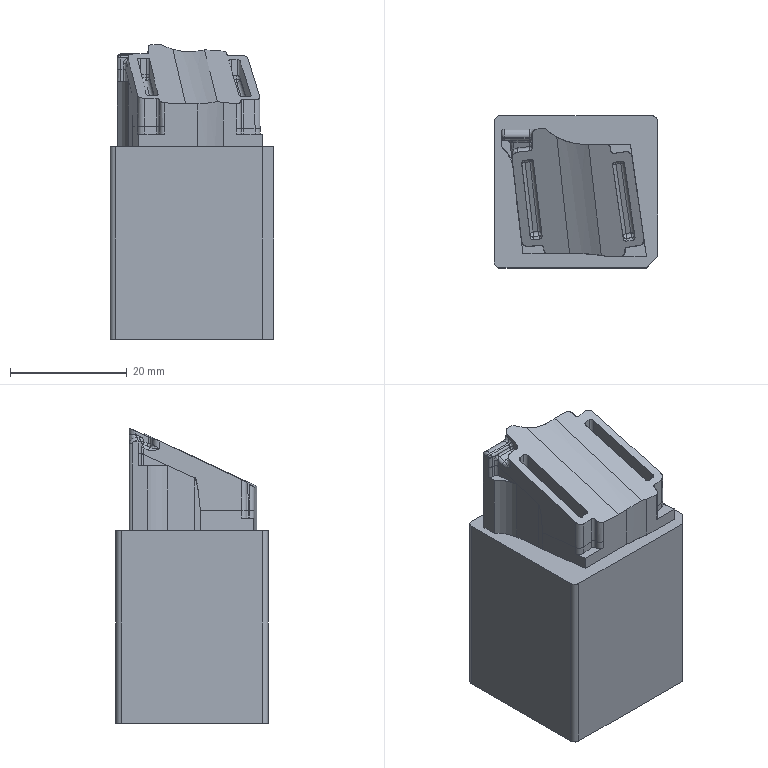NC program | NX | posted with a generic post | part box 28 x 26 x 50.455 mm
Lines 1 to 1159 of 12518:
N10 G17 G21 G94 G90
(ZLEVEL_PROFILE_COPY , TOOL : D0.5)
N12 T00 M6
N14 G54
N16 G17 G0 G90 X-7.188 Y11.048 S0 M3
N18 G43 Z10. H0
N20 Z0.198
N22 G94 G1 Z-0.102 F250.
N24 G3 X-6.499 Y10.968 R3.
N26 G1 X-5.218
N28 X-5.116 Y10.979
N30 X-5.049 Y10.902
N32 X-4.947 Y10.81
N34 G3 X-4.652 Y10.578 R3.
N36 G1 Z0.198
N38 G0 Z0.997
N40 X-4.451 Y10.419
N42 Z0.098
N44 G1 Z-0.202
N46 G2 X-4.773 Y10.658 R3.
N48 X-5.049 Y10.902 R9.75
N50 G1 X-5.116 Y10.979
N52 X-5.218 Y10.968
N54 X-6.5
N56 G2 X-7.189 Y11.048 R3.
N58 G1 Z0.098
N60 G0 Z0.898
N62 X-7.19
N64 Z-0.001
N66 G1 Z-0.301
N68 G3 X-6.5 Y10.968 R3.
N70 G1 X-5.218
N72 X-5.116 Y10.979
N74 X-5.049 Y10.902
N76 G3 X-4.553 Y10.476 R9.75
N78 X-4.22 Y10.244 R3.
N80 G1 Z-0.001
N82 G0 Z0.798
N84 X-3.978 Y10.072
N86 Z-0.1
N88 G1 Z-0.4
N90 G2 X-4.319 Y10.294 R3.
N92 X-5.049 Y10.902 R9.75
N94 G1 X-5.116 Y10.979
N96 X-5.218 Y10.968
N98 X-6.501
N100 G2 X-7.192 Y11.048 R3.
N102 G1 Z-0.1
N104 G0 Z0.699
N106 X-7.193
N108 Z-0.2
N110 G1 Z-0.5
N112 G3 X-6.501 Y10.968 R3.
N114 G1 X-5.218
N116 X-5.116 Y10.979
N118 X-5.049 Y10.902
N120 G3 X-4.07 Y10.112 R9.75
N122 X-3.726 Y9.903 R3.
N124 G1 Z-0.2
N126 G0 Z0.6
N128 X-3.456 Y9.735
N130 Z-0.299
N132 G1 Z-0.599
N134 G2 X-3.81 Y9.935 R3.
N136 X-4.07 Y10.112 R9.75
N138 X-5.049 Y10.902 R9.75
N140 G1 X-5.116 Y10.979
N142 X-5.218 Y10.968
N144 X-6.501
N146 G2 X-7.194 Y11.048 R3.
N148 G1 Z-0.299
N150 G0 Z0.5
N152 Z-0.398
N154 G1 Z-0.698
N156 G3 X-6.502 Y10.968 R3.
N158 G1 X-5.218
N160 X-5.116 Y10.979
N162 X-5.049 Y10.902
N164 G3 X-4.07 Y10.112 R9.75
N166 X-3.531 Y9.759 R9.75
N168 X-3.171 Y9.571 R3.
N170 G1 Z-0.398
N172 G0 Z0.401
N174 X-2.857 Y9.405
N176 Z-0.498
N178 G1 Z-0.798
N180 G2 X-3.233 Y9.584 R3.
N182 X-3.531 Y9.759 R9.75
N184 X-4.07 Y10.112 R9.75
N186 X-5.049 Y10.902 R9.75
N188 G1 X-5.116 Y10.979
N190 X-5.218 Y10.968
N192 X-6.501
N194 G2 X-7.195 Y11.048 R3.
N196 G1 Z-0.498
N198 G0 Z0.302
N200 Z-0.597
N202 G1 Z-0.897
N204 G3 X-6.504 Y10.968 R3.
N206 G1 X-5.218
N208 X-5.116 Y10.979
N210 X-5.049 Y10.902
N212 G3 X-4.07 Y10.112 R9.75
N214 X-3.531 Y9.759 R9.75
N216 X-3.233 Y9.584 R9.75
N218 G1 X-3.232 Y9.583
N220 G3 X-2.901 Y9.405 R9.75
N222 X-2.521 Y9.243 R3.
N224 G1 Z-0.597
N226 G0 Z0.202
N228 X-2.115 Y9.069
N230 Z-0.696
N232 G1 Z-0.996
N234 G2 X-2.52 Y9.22 R3.
N236 X-3.232 Y9.583 R9.75
N238 G1 X-3.233 Y9.584
N240 G2 X-3.531 Y9.759 R9.75
N242 X-4.07 Y10.112 R9.75
N244 X-5.049 Y10.902 R9.75
N246 G1 X-5.116 Y10.979
N248 X-5.218 Y10.968
N250 X-6.501
N252 X-6.506
N254 G2 X-7.198 Y11.048 R3.
N256 G1 Z-0.696
N258 G0 Z0.103
N260 X-7.214 Y11.051
N262 Z-0.796
N264 G1 Z-1.096
N266 G3 X-6.513 Y10.968 R3.
N268 G1 X-6.504
N270 X-5.218
N272 X-5.116 Y10.979
N274 X-5.049 Y10.902
N276 G3 X-4.07 Y10.112 R9.75
N278 X-3.233 Y9.584 R9.75
N280 G1 X-3.232 Y9.583
N282 G3 X-2.52 Y9.22 R9.75
N284 G1 X-2.478 Y9.201
N286 G3 X-2.054 Y9.021 R9.75
N288 X-1.664 Y8.896 R3.
N290 G1 Z-0.796
N292 G0 Z0.004
N294 X-1.126 Y8.713
N296 Z-0.895
N298 G1 Z-1.195
N300 G2 X-1.372 Y8.779 R3.
N302 X-2.054 Y9.021 R9.75
N304 X-2.478 Y9.201 R9.75
N306 G1 X-2.52 Y9.22
N308 G2 X-3.232 Y9.583 R9.75
N310 G1 X-3.233 Y9.584
N312 G2 X-4.07 Y10.112 R9.75
N314 X-5.049 Y10.902 R9.75
N316 G1 X-5.116 Y10.979
N318 X-5.218 Y10.968
N320 X-6.501
N322 X-6.513
N324 X-6.521
N326 G2 X-7.217 Y11.054 R3.
N328 G1 Z-0.895
N330 G0 Z10.
N332 X1.377 Y8.359
N334 Z-0.696
N336 G1 Z-0.996
N338 G3 X1.781 Y8.331 R3.
N340 G1 X3.342
N342 G3 X3.757 Y8.36 R3.
N344 G1 Z-0.696
N346 G0 Z0.103
N348 X5.252
N350 Z-0.796
N352 G1 Z-1.096
N354 G2 X4.837 Y8.331 R3.
N356 G1 X1.548
N358 G2 X1.309 Y8.334 R9.75
N360 X0.889 Y8.374 R3.
N362 G1 Z-0.796
N364 G0 Z0.004
N366 X0.234 Y8.439
N368 Z-0.895
N370 G1 Z-1.195
N372 G3 X0.635 Y8.374 R3.
N374 X1.294 Y8.334 R9.75
N376 G1 X1.309
N378 G3 X1.548 Y8.331 R9.75
N380 G1 X5.128
N382 G2 X5.669 Y8.174 R1.142
N384 G3 X6.037 Y7.99 R3.
N386 G1 Z-0.895
N388 G0 Z-0.096
N390 X6.22 Y7.666
N392 Z-0.994
N394 G1 Z-1.294
N396 G2 X5.901 Y7.985 R3.
N398 G3 X5.129 Y8.331 R0.992
N400 G1 X1.548
N402 G2 X1.309 Y8.334 R9.75
N404 G1 X1.294
N406 G2 X-2.054 Y9.021 R9.75
N408 X-2.478 Y9.201 R9.75
N410 G1 X-2.52 Y9.22
N412 G2 X-3.232 Y9.583 R9.75
N414 G1 X-3.233 Y9.584
N416 G2 X-4.07 Y10.112 R9.75
N418 X-5.049 Y10.902 R9.75
N420 G1 X-5.116 Y10.979
N422 X-5.218 Y10.968
N424 X-6.501
N426 X-6.513
N428 X-6.536
N430 X-6.538
N432 G2 X-7.255 Y11.052 R3.
N434 G1 Z-0.994
N436 G0 Z-0.195
N438 X-7.261 Y11.057
N440 Z-1.094
N442 G1 Z-1.394
N444 G3 X-6.559 Y10.968 R3.
N446 G1 X-6.541
N448 X-6.536
N450 X-6.513
N452 X-6.504
N454 X-5.218
N456 X-5.116 Y10.979
N458 X-5.049 Y10.902
N460 G3 X-4.07 Y10.112 R9.75
N462 X-3.233 Y9.584 R9.75
N464 G1 X-3.232 Y9.583
N466 G3 X-2.52 Y9.22 R9.75
N468 G1 X-2.478 Y9.201
N470 G3 X-2.054 Y9.021 R9.75
N472 X1.294 Y8.334 R9.75
N474 G1 X1.309
N476 G3 X1.548 Y8.331 R9.75
N478 G1 X5.129
N480 G2 X5.438 Y8.288 R0.992
N482 X6.002 Y7.856 R1.008
N484 G3 X6.346 Y7.563 R3.
N486 G1 Z-1.094
N488 G0 Z-0.294
N490 X6.24 Y6.997
N492 Z-1.193
N494 G1 Z-1.493
N496 G2 X6.166 Y7.405 R3.
N498 G3 X6.096 Y7.681 R1.042
N500 G1 X6.091 Y7.786
N502 X6.008 Y7.851
N504 X5.947 Y7.936
N506 G3 X5.438 Y8.288 R1.008
N508 X5.129 Y8.331 R0.992
N510 G1 X1.548
N512 G2 X1.309 Y8.334 R9.75
N514 G1 X1.294
N516 G2 X-2.054 Y9.021 R9.75
N518 X-2.478 Y9.201 R9.75
N520 G1 X-2.52 Y9.22
N522 G2 X-3.232 Y9.583 R9.75
N524 G1 X-3.233 Y9.584
N526 G2 X-4.07 Y10.112 R9.75
N528 X-5.049 Y10.902 R9.75
N530 G1 X-5.116 Y10.979
N532 X-5.218 Y10.968
N534 X-6.501
N536 X-6.513
N538 X-6.536
N540 X-6.541
N542 X-6.587
N544 G2 X-7.338 Y11.052 R3.
N546 G1 Z-1.193
N548 G0 Z-0.394
N550 X-7.351 Y11.065
N552 Z-1.292
N554 G1 Z-1.592
N556 G3 X-6.621 Y10.968 R3.
N558 G1 X-6.591
N560 X-6.541
N562 X-6.536
N564 X-6.513
N566 X-6.504
N568 X-5.218
N570 X-5.116 Y10.979
N572 X-5.049 Y10.902
N574 G3 X-4.07 Y10.112 R9.75
N576 X-3.233 Y9.584 R9.75
N578 G1 X-3.232 Y9.583
N580 G3 X-2.52 Y9.22 R9.75
N582 G1 X-2.478 Y9.201
N584 G3 X-2.054 Y9.021 R9.75
N586 X1.294 Y8.334 R9.75
N588 G1 X1.309
N590 G3 X1.548 Y8.331 R9.75
N592 G1 X5.129
N594 G2 X5.438 Y8.288 R0.992
N596 X5.834 Y8.061 R1.008
N598 X6.022 Y7.835 R1.05
N600 G1 X6.09 Y7.789
N602 Y7.707
N604 G2 X6.18 Y7.279 R1.05
N606 G1 Y7.118
N608 G3 X6.204 Y6.733 R3.
N610 G1 Z-1.292
N612 G0 Z-0.493
N614 X6.218 Y6.555
N616 Z-1.391
N618 G1 Z-1.691
N620 G2 X6.18 Y7.04 R3.
N622 G1 X6.181 Y7.279
N624 G3 X6.089 Y7.71 R1.05
N626 G1 X6.09 Y7.789
N628 X6.024 Y7.833
N630 G3 X5.817 Y8.076 R1.05
N632 X5.438 Y8.288 R1.008
N634 X5.129 Y8.331 R0.992
N636 G1 X1.548
N638 G2 X1.309 Y8.334 R9.75
N640 G1 X1.294
N642 G2 X-2.054 Y9.021 R9.75
N644 X-2.478 Y9.201 R9.75
N646 G1 X-2.52 Y9.22
N648 G2 X-3.232 Y9.583 R9.75
N650 G1 X-3.233 Y9.584
N652 G2 X-4.07 Y10.112 R9.75
N654 X-5.049 Y10.902 R9.75
N656 G1 X-5.116 Y10.979
N658 X-5.218 Y10.968
N660 X-6.501
N662 X-6.513
N664 X-6.536
N666 X-6.541
N668 X-6.591
N670 X-6.66
N672 G2 X-7.421 Y11.049 R3.
N674 G1 Z-1.391
N676 G0 Z-0.592
N678 X-7.471 Y11.066
N680 Z-1.491
N682 G1 Z-1.791
N684 G3 X-6.71 Y10.968 R3.
N686 G1 X-6.676
N688 X-6.591
N690 X-6.541
N692 X-6.536
N694 X-6.513
N696 X-6.504
N698 X-5.218
N700 X-5.116 Y10.979
N702 X-5.049 Y10.902
N704 G3 X-4.07 Y10.112 R9.75
N706 X-3.233 Y9.584 R9.75
N708 G1 X-3.232 Y9.583
N710 G3 X-2.52 Y9.22 R9.75
N712 G1 X-2.478 Y9.201
N714 G3 X-2.054 Y9.021 R9.75
N716 X1.294 Y8.334 R9.75
N718 G1 X1.309
N720 G3 X1.548 Y8.331 R9.75
N722 G1 X5.129
N724 G2 X5.438 Y8.288 R0.992
N726 X5.801 Y8.09 R1.008
N728 X6.026 Y7.831 R1.05
N730 G1 X6.09 Y7.789
N732 X6.088 Y7.713
N734 G2 X6.181 Y7.279 R1.05
N736 G1 Y7.083
N738 G3 X6.247 Y6.885 R0.526
N740 X6.482 Y6.537 R3.
N742 G1 Z-1.491
N744 G0 Z-0.691
N746 X6.785 Y6.691
N748 Z-1.59
N750 G1 Z-1.89
N752 G2 X6.37 Y6.811 R3.
N754 G1 X6.267 Y6.836
N756 X6.223 Y6.932
N758 X6.181 Y7.079
N760 Y7.083
N762 X6.182 Y7.279
N764 G3 X6.087 Y7.716 R1.05
N766 G1 X6.028 Y7.829
N768 G3 X5.784 Y8.104 R1.05
N770 X5.438 Y8.288 R1.008
N772 X5.129 Y8.331 R0.992
N774 G1 X1.548
N776 G2 X1.309 Y8.334 R9.75
N778 G1 X1.294
N780 G2 X-2.054 Y9.021 R9.75
N782 X-2.478 Y9.201 R9.75
N784 G1 X-2.52 Y9.22
N786 G2 X-3.232 Y9.583 R9.75
N788 G1 X-3.233 Y9.584
N790 G2 X-4.07 Y10.112 R9.75
N792 X-5.049 Y10.902 R9.75
N794 G1 X-5.116 Y10.979
N796 X-5.218 Y10.968
N798 X-6.501
N800 X-6.513
N802 X-6.536
N804 X-6.541
N806 X-6.591
N808 X-6.676
N810 X-6.764
N812 G2 X-7.545 Y11.071 R3.
N814 G1 Z-1.59
N816 G0 Z-0.791
N818 X-7.645 Y11.08
N820 Z-1.689
N822 G1 Z-1.989
N824 G3 X-6.832 Y10.968 R3.
N826 G1 X-6.764
N828 X-6.676
N830 X-6.591
N832 X-6.541
N834 X-6.536
N836 X-6.513
N838 X-6.504
N840 X-5.218
N842 X-5.116 Y10.979
N844 X-5.049 Y10.902
N846 G3 X-4.07 Y10.112 R9.75
N848 X-3.233 Y9.584 R9.75
N850 G1 X-3.232 Y9.583
N852 G3 X-2.52 Y9.22 R9.75
N854 G1 X-2.478 Y9.201
N856 G3 X-2.054 Y9.021 R9.75
N858 X1.294 Y8.334 R9.75
N860 G1 X1.309
N862 G3 X1.548 Y8.331 R9.75
N864 G1 X5.129
N866 G2 X5.438 Y8.288 R0.992
N868 X5.766 Y8.118 R1.008
N870 X6.03 Y7.826 R1.05
N872 G1 X6.086 Y7.72
N874 G2 X6.182 Y7.279 R1.05
N876 G1 Y7.083
N878 X6.181 Y7.078
N880 X6.223 Y6.932
N882 X6.267 Y6.836
N884 X6.37 Y6.811
N886 X6.389 Y6.804
N888 X6.457 Y6.799
N890 X8.394 Y7.08
N892 X8.735 Y7.078
N894 X8.859 Y7.057
N896 X8.882 Y7.051
N898 X9.063 Y6.984
N900 G3 X9.481 Y6.863 R3.
N902 G1 Z-1.689
N904 G0 Z-0.89
N906 X9.751 Y6.474
N908 Z-1.789
N910 G1 Z-2.089
N912 G2 X9.426 Y6.744 R3.
N914 G3 X9.121 Y6.959 R1.249
N916 G1 X9.083 Y6.977
N918 G3 X8.895 Y7.046 R1.249
N920 G1 X8.882 Y7.051
N922 X8.859 Y7.057
N924 X8.841 Y7.06
N926 G3 X8.395 Y7.08 R1.249
N928 G1 X6.455 Y6.8
N930 X6.388 Y6.805
N932 X6.37 Y6.811
N934 X6.267 Y6.836
N936 X6.223 Y6.932
N938 X6.182 Y7.076
N940 Y7.083
N942 X6.183 Y7.279
N944 G3 X6.085 Y7.723 R1.05
N946 G1 X6.032 Y7.823
N948 G3 X5.748 Y8.132 R1.05
N950 X5.438 Y8.288 R1.008
N952 X5.129 Y8.331 R0.992
N954 G1 X1.548
N956 G2 X1.309 Y8.334 R9.75
N958 G1 X1.294
N960 G2 X-2.054 Y9.021 R9.75
N962 X-2.478 Y9.201 R9.75
N964 G1 X-2.52 Y9.22
N966 G2 X-3.232 Y9.583 R9.75
N968 G1 X-3.233 Y9.584
N970 G2 X-4.07 Y10.112 R9.75
N972 X-5.049 Y10.902 R9.75
N974 G1 X-5.116 Y10.979
N976 X-5.218 Y10.968
N978 X-6.501
N980 X-6.513
N982 X-6.536
N984 X-6.541
N986 X-6.591
N988 X-6.676
N990 X-6.908
N992 G2 X-7.78 Y11.097 R3.
N994 G1 Z-1.789
N996 G0 Z-0.989
N998 X-7.947 Y11.122
N1000 Z-1.888
N1002 G1 Z-2.188
N1004 G3 X-6.998 Y10.968 R3.
N1006 G1 X-6.676
N1008 X-6.591
N1010 X-6.541
N1012 X-6.536
N1014 X-6.513
N1016 X-6.504
N1018 X-5.218
N1020 X-5.116 Y10.979
N1022 X-5.049 Y10.902
N1024 G3 X-4.07 Y10.112 R9.75
N1026 X-3.233 Y9.584 R9.75
N1028 G1 X-3.232 Y9.583
N1030 G3 X-2.52 Y9.22 R9.75
N1032 G1 X-2.478 Y9.201
N1034 G3 X-2.054 Y9.021 R9.75
N1036 X1.294 Y8.334 R9.75
N1038 G1 X1.309
N1040 G3 X1.548 Y8.331 R9.75
N1042 G1 X5.129
N1044 G2 X5.438 Y8.288 R0.992
N1046 X5.73 Y8.145 R1.008
N1048 X6.034 Y7.821 R1.05
N1050 G1 X6.084 Y7.727
N1052 G2 X6.183 Y7.279 R1.05
N1054 G1 Y7.083
N1056 X6.182 Y7.073
N1058 X6.223 Y6.932
N1060 X6.267 Y6.836
N1062 X6.37 Y6.811
N1064 X6.387 Y6.805
N1066 X6.453 Y6.8
N1068 X8.395 Y7.081
N1070 G2 X9.619 Y6.527 R1.204
N1072 G3 X9.874 Y6.173 R3.
N1074 G1 Z-1.888
N1076 G0 Z-1.089
N1078 X9.894 Y5.833
N1080 Z-1.987
N1082 G1 Z-2.287
N1084 G2 X9.763 Y6.221 R3.
N1086 G1 X9.755 Y6.252
N1088 X9.712 Y6.357
N1090 G3 X9.332 Y6.846 R1.222
N1092 X8.475 Y7.092 R1.204
N1094 G1 X8.396 Y7.082
N1096 X6.451 Y6.8
N1098 X6.387 Y6.805
N1100 X6.37 Y6.811
N1102 X6.267 Y6.836
N1104 X6.223 Y6.932
N1106 X6.182 Y7.071
N1108 X6.183 Y7.083
N1110 X6.184 Y7.279
N1112 G3 X6.083 Y7.731 R1.05
N1114 G1 X6.037 Y7.817
N1116 G3 X5.711 Y8.158 R1.05
N1118 X5.438 Y8.288 R1.008
N1120 X5.129 Y8.331 R0.992
N1122 G1 X1.548
N1124 G2 X1.309 Y8.334 R9.75
N1126 G1 X1.294
N1128 G2 X-2.054 Y9.021 R9.75
N1130 X-2.478 Y9.201 R9.75
N1132 G1 X-2.52 Y9.22
N1134 G2 X-3.232 Y9.583 R9.75
N1136 G1 X-3.233 Y9.584
N1138 G2 X-4.07 Y10.112 R9.75
N1140 X-5.049 Y10.902 R9.75
N1142 G1 X-5.116 Y10.979
N1144 X-5.218 Y10.968
N1146 X-6.501
N1148 X-6.513
N1150 X-6.536
N1152 X-6.541
N1154 X-6.591
N1156 X-6.676
N1158 X-7.109
N1160 G2 X-8.164 Y11.159 R3.
N1162 G1 Z-1.987
N1164 G0 Z-1.188
N1166 X-8.372 Y11.189
N1168 Z-2.087
N1170 G1 Z-2.387
N1172 G3 X-7.241 Y10.968 R3.
N1174 G1 X-6.676
N1176 X-6.591
N1178 X-6.541
N1180 X-6.536
N1182 X-6.513
N1184 X-6.504
N1186 X-5.218
N1188 X-5.116 Y10.979
N1190 X-5.049 Y10.902
N1192 G3 X-4.07 Y10.112 R9.75
N1194 X-3.233 Y9.584 R9.75
N1196 G1 X-3.232 Y9.583
N1198 G3 X-2.52 Y9.22 R9.75
N1200 G1 X-2.478 Y9.201
N1202 G3 X-2.054 Y9.021 R9.75
N1204 X1.294 Y8.334 R9.75
N1206 G1 X1.309
N1208 G3 X1.548 Y8.331 R9.75
N1210 G1 X5.129
N1212 G2 X5.438 Y8.288 R0.992
N1214 X5.692 Y8.171 R1.008
N1216 X6.039 Y7.814 R1.05
N1218 G1 X6.081 Y7.735
N1220 G2 X6.184 Y7.279 R1.05
N1222 G1 Y7.083
N1224 X6.183 Y7.069
N1226 X6.223 Y6.932
N1228 X6.267 Y6.836
N1230 X6.37 Y6.811
N1232 X6.386 Y6.805
N1234 X6.449 Y6.8
N1236 X8.396 Y7.082
N1238 X8.464 Y7.091
N1240 X8.475 Y7.092
N1242 G2 X9.332 Y6.846 R1.204
N1244 X9.693 Y6.4 R1.222
N1246 G1 X9.722 Y6.335
N1248 X9.755 Y6.254
N1250 X9.761 Y6.231
N1252 X9.763 Y6.221
N1254 X9.765 Y6.214
N1256 X9.813 Y6.021
N1258 X9.817 Y5.993
N1260 G3 X9.904 Y5.586 R3.
N1262 G1 Z-2.087
N1264 G0 Z-1.287
N1266 X9.933 Y5.37
N1268 Z-2.186
N1270 G1 Z-2.486
N1272 G2 X9.85 Y5.766 R3.
N1274 G1 X9.813 Y6.021
N1276 X9.755 Y6.253
N1278 Y6.255
N1280 X9.731 Y6.314
N1282 X9.696 Y6.394
N1284 X9.693 Y6.4
N1286 G3 X9.332 Y6.846 R1.222
N1288 X8.475 Y7.092 R1.204
N1290 G1 X8.465 Y7.091
N1292 X8.397 Y7.083
N1294 X6.447 Y6.8
N1296 X6.386 Y6.806
N1298 X6.37 Y6.811
N1300 X6.267 Y6.836
N1302 X6.223 Y6.932
N1304 X6.183 Y7.067
N1306 X6.184 Y7.083
N1308 X6.185 Y7.279
N1310 G3 X6.079 Y7.74 R1.05
N1312 G1 X6.042 Y7.81
N1314 G3 X5.672 Y8.183 R1.05
N1316 X5.438 Y8.288 R1.008
N1318 X5.129 Y8.331 R0.992
N1320 G1 X1.548
N1322 G2 X1.309 Y8.334 R9.75
N1324 G1 X1.294
N1326 G2 X-2.054 Y9.021 R9.75
N1328 X-2.478 Y9.201 R9.75
N1330 G1 X-2.52 Y9.22
N1332 G2 X-3.232 Y9.583 R9.75
N1334 G1 X-3.233 Y9.584
N1336 G2 X-4.07 Y10.112 R9.75
N1338 X-5.049 Y10.902 R9.75
N1340 G1 X-5.116 Y10.979
N1342 X-5.218 Y10.968
N1344 X-6.501
N1346 X-6.513
N1348 X-6.536
N1350 X-6.541
N1352 X-6.591
N1354 X-6.676
N1356 X-7.415
N1358 G2 X-8.592 Y11.208 R3.
N1360 G1 Z-2.186
N1362 G0 Z-1.387
N1364 X-8.903 Y11.217
N1366 Z-2.285
N1368 G1 Z-2.585
N1370 G3 X-7.705 Y10.968 R3.
N1372 G1 X-6.676
N1374 X-6.591
N1376 X-6.541
N1378 X-6.536
N1380 X-6.513
N1382 X-6.504
N1384 X-5.218
N1386 X-5.116 Y10.979
N1388 X-5.049 Y10.902
N1390 G3 X-4.07 Y10.112 R9.75
N1392 X-3.233 Y9.584 R9.75
N1394 G1 X-3.232 Y9.583
N1396 G3 X-2.52 Y9.22 R9.75
N1398 G1 X-2.478 Y9.201
N1400 G3 X-2.054 Y9.021 R9.75
N1402 X1.294 Y8.334 R9.75
N1404 G1 X1.309
N1406 G3 X1.548 Y8.331 R9.75
N1408 G1 X5.129
N1410 G2 X5.438 Y8.288 R0.992
N1412 X5.652 Y8.195 R1.008
N1414 X6.045 Y7.806 R1.05
N1416 G1 X6.077 Y7.745
N1418 G2 X6.185 Y7.279 R1.05
N1420 G1 Y7.083
N1422 X6.184 Y7.064
N1424 X6.223 Y6.932
N1426 X6.26 Y6.842
N1428 X6.354 Y6.817
N1430 X6.429 Y6.804
N1432 X6.51 Y6.81
N1434 X8.397 Y7.083
N1436 X8.466 Y7.091
N1438 X8.475 Y7.092
N1440 G2 X9.332 Y6.846 R1.204
N1442 X9.693 Y6.4 R1.222
N1444 G1 X9.696 Y6.394
N1446 X9.699 Y6.388
N1448 X9.741 Y6.292
N1450 X9.755 Y6.256
N1452 X9.812 Y6.035
N1454 X9.878 Y5.57
N1456 G3 X9.949 Y5.219 R3.
N1458 G1 Z-2.285
N1460 G0 Z10.
N1462 X-10.386 Y8.2
N1464 Z-2.087
N1466 G1 Z-2.387
N1468 G3 X-11.252 Y8.475 R1.5
N1470 G1 X-12.311
N1472 G2 X-12.929 Y8.878 R0.78
N1474 G1 X-12.934 Y8.88
N1476 X-12.974 Y8.974
N1478 X-12.986 Y9.022
N1480 X-12.999 Y9.073
N1482 X-13.015 Y9.153
N1484 Y9.216
N1486 Y9.259
N1488 Y9.96
N1490 X-13.016 Y10.11
N1492 X-13.015 Y10.157
N1494 G3 X-13.051 Y10.774 R3.
N1496 G1 Z-2.087
N1498 G0 Z-1.287
N1500 X-13.074 Y10.792
N1502 Z-2.186
N1504 G1 Z-2.486
N1506 G2 X-13.015 Y10.197 R3.
N1508 G1 Y10.159
N1510 X-13.016 Y10.11
N1512 X-13.015 Y9.96
N1514 Y9.259
N1516 Y9.216
N1518 Y9.152
N1520 X-12.999 Y9.072
N1522 X-12.986 Y9.022
N1524 X-12.974 Y8.974
N1526 X-12.934 Y8.88
N1528 X-12.929 Y8.877
N1530 G3 X-12.544 Y8.532 R0.769
N1532 X-12.311 Y8.475 R0.78
N1534 G1 X-12.279
N1536 X-12.265
N1538 X-11.381
N1540 Z-2.186
N1542 G0 Z-1.387
N1544 X-10.81 Y8.088
N1546 Z-2.285
N1548 G1 Z-2.585
N1550 G3 X-11.469 Y8.475 R0.982
N1552 G1 X-12.265 Y8.474
N1554 X-12.288 Y8.475
N1556 X-12.311
N1558 X-12.444 Y8.498
N1560 G2 X-12.929 Y8.877 R0.766
N1562 G1 X-12.934 Y8.88
N1564 X-12.974 Y8.974
N1566 X-12.986 Y9.022
N1568 X-12.999 Y9.071
N1570 X-13.015 Y9.152
N1572 Y9.216
N1574 Y9.259
N1576 Y9.96
N1578 X-13.016 Y10.11
N1580 X-13.015 Y10.159
N1582 Y10.197
N1584 Y10.208
N1586 Y10.216
N1588 G3 X-13.073 Y10.805 R3.
N1590 G1 Z-2.285
N1592 G0 Z0.6
N1594 X9.995 Y4.952
N1596 Z-2.385
N1598 G1 Z-2.685
N1600 G2 X9.908 Y5.358 R3.
N1602 G1 X9.809 Y6.061
N1604 X9.755 Y6.257
N1606 X9.75 Y6.27
N1608 X9.702 Y6.381
N1610 X9.699 Y6.388
N1612 X9.696 Y6.394
N1614 X9.693 Y6.4
N1616 G3 X9.332 Y6.846 R1.222
N1618 X8.475 Y7.092 R1.204
N1620 G1 X8.468 Y7.091
N1622 X8.397 Y7.084
N1624 X6.524 Y6.813
N1626 X6.429 Y6.804
N1628 X6.354 Y6.817
N1630 X6.26 Y6.842
N1632 X6.223 Y6.932
N1634 X6.184 Y7.062
N1636 X6.185 Y7.083
N1638 X6.186 Y7.279
N1640 G3 X6.075 Y7.751 R1.05
N1642 G1 X6.049 Y7.8
N1644 G3 X5.632 Y8.206 R1.05
N1646 X5.438 Y8.288 R1.008
N1648 X5.129 Y8.331 R0.992
N1650 G1 X1.548
N1652 G2 X1.309 Y8.334 R9.75
N1654 G1 X1.294
N1656 G2 X-2.054 Y9.021 R9.75
N1658 X-2.478 Y9.201 R9.75
N1660 G1 X-2.52 Y9.22
N1662 G2 X-3.232 Y9.583 R9.75
N1664 G1 X-3.233 Y9.584
N1666 G2 X-4.07 Y10.112 R9.75
N1668 X-5.049 Y10.902 R9.75
N1670 G1 X-5.116 Y10.979
N1672 X-5.218 Y10.968
N1674 X-6.501
N1676 X-6.513
N1678 X-6.536
N1680 X-6.541
N1682 X-6.591
N1684 X-6.676
N1686 X-12.265
N1688 G3 X-13.015 Y10.218 R0.75
N1690 G1 Y10.216
N1692 Y10.208
N1694 Y10.197
N1696 Y10.159
N1698 X-13.016 Y10.11
N1700 X-13.015 Y9.96
N1702 Y9.259
N1704 Y9.216
N1706 Y9.151
N1708 X-12.999 Y9.071
N1710 X-12.986 Y9.021
N1712 X-12.974 Y8.974
N1714 X-12.934 Y8.88
N1716 X-12.929 Y8.877
N1718 G3 X-12.41 Y8.49 R0.766
N1720 G1 X-12.311 Y8.475
N1722 X-12.295
N1724 X-12.265 Y8.474
N1726 X-11.574
N1728 Z-2.385
N1730 G0 Z-0.989
N1732 X-13.075 Y8.642
N1734 Z-2.484
N1736 G1 Z-2.784
N1738 G3 X-11.655 Y8.474 R3.
N1740 G1 X-12.265
N1742 X-12.301 Y8.475
N1744 X-12.311
N1746 X-12.376 Y8.483
N1748 G2 X-12.929 Y8.877 R0.766
N1750 G1 X-12.934 Y8.88
N1752 X-12.974 Y8.974
N1754 X-12.986 Y9.021
N1756 X-12.998 Y9.061
N1758 X-12.999 Y9.07
N1760 X-13.015 Y9.151
N1762 Y9.216
N1764 Y9.259
N1766 Y9.96
N1768 X-13.016 Y10.11
N1770 X-13.015 Y10.159
N1772 Y10.197
N1774 Y10.208
N1776 Y10.216
N1778 Y10.217
N1780 G2 X-12.265 Y10.968 R0.75
N1782 G1 X-6.676
N1784 X-6.591
N1786 X-6.541
N1788 X-6.536
N1790 X-6.513
N1792 X-6.504
N1794 X-5.218
N1796 X-5.116 Y10.979
N1798 X-5.049 Y10.902
N1800 G3 X-4.07 Y10.112 R9.75
N1802 X-3.233 Y9.584 R9.75
N1804 G1 X-3.232 Y9.583
N1806 G3 X-2.52 Y9.22 R9.75
N1808 G1 X-2.478 Y9.201
N1810 G3 X-2.054 Y9.021 R9.75
N1812 X1.294 Y8.334 R9.75
N1814 G1 X1.309
N1816 G3 X1.548 Y8.331 R9.75
N1818 G1 X5.129
N1820 G2 X5.438 Y8.288 R0.992
N1822 G1 X5.612 Y8.217
N1824 G2 X6.053 Y7.793 R1.05
N1826 G1 X6.071 Y7.76
N1828 G2 X6.186 Y7.279 R1.05
N1830 G1 Y7.083
N1832 X6.184 Y7.06
N1834 X6.223 Y6.932
N1836 X6.26 Y6.842
N1838 X6.354 Y6.817
N1840 X6.429 Y6.804
N1842 X6.544 Y6.816
N1844 X8.398 Y7.085
N1846 X8.574 Y7.097
N1848 G2 X9.332 Y6.846 R1.204
N1850 G1 X9.465 Y6.727
N1852 G2 X9.809 Y6.062 R1.25
N1854 G1 Y6.059
N1856 X9.815 Y6.023
N1858 X9.939 Y5.147
N1860 G3 X10.026 Y4.74 R3.
N1862 G1 Z-2.484
N1864 G0 Z-1.685
N1866 X10.056 Y4.529
N1868 Z-2.583
N1870 G1 Z-2.883
N1872 G2 X9.97 Y4.935 R3.
N1874 G1 X9.815 Y6.024
N1876 G3 X9.4 Y6.789 R1.25
N1878 G1 X9.332 Y6.846
N1880 G3 X8.617 Y7.097 R1.204
N1882 X8.398 Y7.085 R1.25
N1884 G1 X6.556 Y6.818
N1886 X6.429 Y6.804
N1888 X6.354 Y6.817
N1890 X6.26 Y6.842
N1892 X6.223 Y6.932
N1894 X6.185 Y7.058
N1896 X6.186 Y7.083
N1898 X6.187 Y7.279
N1900 G3 X5.591 Y8.228 R1.05
N1902 G1 X5.438 Y8.288
N1904 G3 X5.129 Y8.331 R0.992
N1906 G1 X1.548
N1908 G2 X1.309 Y8.334 R9.75
N1910 G1 X1.294
N1912 G2 X-2.054 Y9.021 R9.75
N1914 X-2.478 Y9.201 R9.75
N1916 G1 X-2.52 Y9.22
N1918 G2 X-3.232 Y9.583 R9.75
N1920 G1 X-3.233 Y9.584
N1922 G2 X-4.07 Y10.112 R9.75
N1924 X-5.049 Y10.902 R9.75
N1926 G1 X-5.116 Y10.979
N1928 X-5.218 Y10.968
N1930 X-6.501
N1932 X-6.513
N1934 X-6.536
N1936 X-6.541
N1938 X-6.591
N1940 X-6.676
N1942 X-12.265
N1944 G3 X-13.015 Y10.218 R0.75
N1946 G1 Y10.216
N1948 Y10.208
N1950 Y10.197
N1952 Y10.159
N1954 X-13.016 Y10.11
N1956 X-13.015 Y9.96
N1958 Y9.259
N1960 Y9.216
N1962 Y9.15
N1964 X-12.999 Y9.07
N1966 X-12.998 Y9.061
N1968 X-12.986 Y9.021
N1970 X-12.974 Y8.974
N1972 X-12.934 Y8.88
N1974 X-12.929 Y8.877
N1976 G3 X-12.343 Y8.479 R0.766
N1978 G1 X-12.311 Y8.475
N1980 X-12.306
N1982 X-12.265 Y8.473
N1984 X-11.69
N1986 Z-2.583
N1988 G0 Z-1.188
N1990 X-12.984 Y8.533
N1992 Z-2.683
N1994 G1 Z-2.983
N1996 G3 X-11.724 Y8.473 R3.
N1998 G1 X-12.265
N2000 G2 X-12.929 Y8.877 R0.766
N2002 G1 X-12.934 Y8.88
N2004 X-12.974 Y8.974
N2006 X-12.986 Y9.021
N2008 X-12.998 Y9.061
N2010 X-12.999 Y9.07
N2012 X-13.015 Y9.15
N2014 Y9.216
N2016 Y9.259
N2018 Y9.96
N2020 X-13.016 Y10.11
N2022 X-13.015 Y10.159
N2024 Y10.197
N2026 Y10.208
N2028 Y10.216
N2030 Y10.217
N2032 G2 X-12.265 Y10.968 R0.75
N2034 G1 X-6.676
N2036 X-6.591
N2038 X-6.541
N2040 X-6.536
N2042 X-6.513
N2044 X-6.504
N2046 X-5.218
N2048 X-5.116 Y10.979
N2050 X-5.049 Y10.902
N2052 G3 X-4.07 Y10.112 R9.75
N2054 X-3.233 Y9.584 R9.75
N2056 G1 X-3.232 Y9.583
N2058 G3 X-2.52 Y9.22 R9.75
N2060 G1 X-2.478 Y9.201
N2062 G3 X-2.054 Y9.021 R9.75
N2064 X1.294 Y8.334 R9.75
N2066 G1 X1.309
N2068 G3 X1.548 Y8.331 R9.75
N2070 G1 X5.129
N2072 G2 X5.438 Y8.288 R0.992
N2074 G1 X5.57 Y8.238
N2076 G2 X6.187 Y7.279 R1.05
N2078 G1 Y7.083
N2080 X6.185 Y7.056
N2082 X6.223 Y6.932
N2084 X6.26 Y6.842
N2086 X6.354 Y6.817
N2088 X6.429 Y6.804
N2090 X6.556 Y6.819
N2092 X8.399 Y7.086
N2094 G2 X8.667 Y7.095 R1.25
N2096 X9.321 Y6.854 R1.204
N2098 X9.815 Y6.024 R1.25
N2100 G1 X10. Y4.724
N2102 G3 X10.087 Y4.317 R3.
N2104 G1 Z-2.683
N2106 G0 Z-1.883
N2108 X10.118 Y4.106
N2110 Z-2.782
N2112 G1 Z-3.082
N2114 G2 X10.031 Y4.512 R3.
N2116 G1 X9.816 Y6.025
N2118 G3 X9.261 Y6.897 R1.25
N2120 X8.73 Y7.09 R1.204
N2122 X8.399 Y7.086 R1.25
N2124 G1 X6.556 Y6.819
N2126 X6.429 Y6.804
N2128 X6.405 Y6.806
N2130 X6.354 Y6.817
N2132 X6.26 Y6.842
N2134 X6.223 Y6.932
N2136 X6.185 Y7.054
N2138 X6.188 Y7.083
N2140 Y7.279
N2142 G3 X5.548 Y8.248 R1.05
N2144 G1 X5.438 Y8.288
N2146 G3 X5.129 Y8.331 R0.992
N2148 G1 X1.548
N2150 G2 X1.309 Y8.334 R9.75
N2152 G1 X1.294
N2154 G2 X-2.054 Y9.021 R9.75
N2156 X-2.478 Y9.201 R9.75
N2158 G1 X-2.52 Y9.22
N2160 G2 X-3.232 Y9.583 R9.75
N2162 G1 X-3.233 Y9.584
N2164 G2 X-4.07 Y10.112 R9.75
N2166 X-5.049 Y10.902 R9.75
N2168 G1 X-5.116 Y10.979
N2170 X-5.218 Y10.968
N2172 X-6.501
N2174 X-6.513
N2176 X-6.536
N2178 X-6.541
N2180 X-6.591
N2182 X-6.676
N2184 X-12.265
N2186 G3 X-13.015 Y10.218 R0.75
N2188 G1 Y10.216
N2190 Y10.208
N2192 Y10.197
N2194 Y10.159
N2196 X-13.016 Y10.11
N2198 X-13.015 Y9.96
N2200 Y9.259
N2202 Y9.216
N2204 Y9.15
N2206 X-12.999 Y9.07
N2208 X-12.998 Y9.061
N2210 X-12.987 Y9.023
N2212 X-12.986 Y9.021
N2214 X-12.974 Y8.974
N2216 X-12.934 Y8.88
N2218 X-12.929 Y8.877
N2220 G3 X-12.265 Y8.473 R0.764
N2222 G1 X-11.708
N2224 Z-2.782
N2226 G0 Z-1.983
N2228 X-11.811 Y8.222
N2230 Z-2.881
N2232 G1 Z-3.181
N2234 G3 X-11.708 Y8.472 R3.
N2236 G1 X-12.265
N2238 G2 X-12.929 Y8.877 R0.764
N2240 G1 X-12.934 Y8.88
N2242 X-12.974 Y8.974
N2244 X-12.986 Y9.021
N2246 X-12.987 Y9.025
N2248 X-12.998 Y9.061
N2250 X-12.999 Y9.069
N2252 X-13.015 Y9.15
N2254 Y9.216
N2256 Y9.259
N2258 Y9.96
N2260 X-13.016 Y10.11
N2262 X-13.015 Y10.159
N2264 Y10.197
N2266 Y10.208
N2268 Y10.216
N2270 Y10.217
N2272 G2 X-12.265 Y10.968 R0.75
N2274 G1 X-6.676
N2276 X-6.591
N2278 X-6.541
N2280 X-6.536
N2282 X-6.513
N2284 X-6.504
N2286 X-5.218
N2288 X-5.116 Y10.979
N2290 X-5.049 Y10.902
N2292 G3 X-4.07 Y10.112 R9.75
N2294 X-3.233 Y9.584 R9.75
N2296 G1 X-3.232 Y9.583
N2298 G3 X-2.52 Y9.22 R9.75
N2300 G1 X-2.478 Y9.201
N2302 G3 X-2.054 Y9.021 R9.75
N2304 X1.294 Y8.334 R9.75
N2306 G1 X1.309
N2308 G3 X1.548 Y8.331 R9.75
N2310 G1 X5.129
N2312 G2 X5.438 Y8.288 R0.992
N2314 G1 X5.527 Y8.257
N2316 G2 X6.189 Y7.279 R1.05